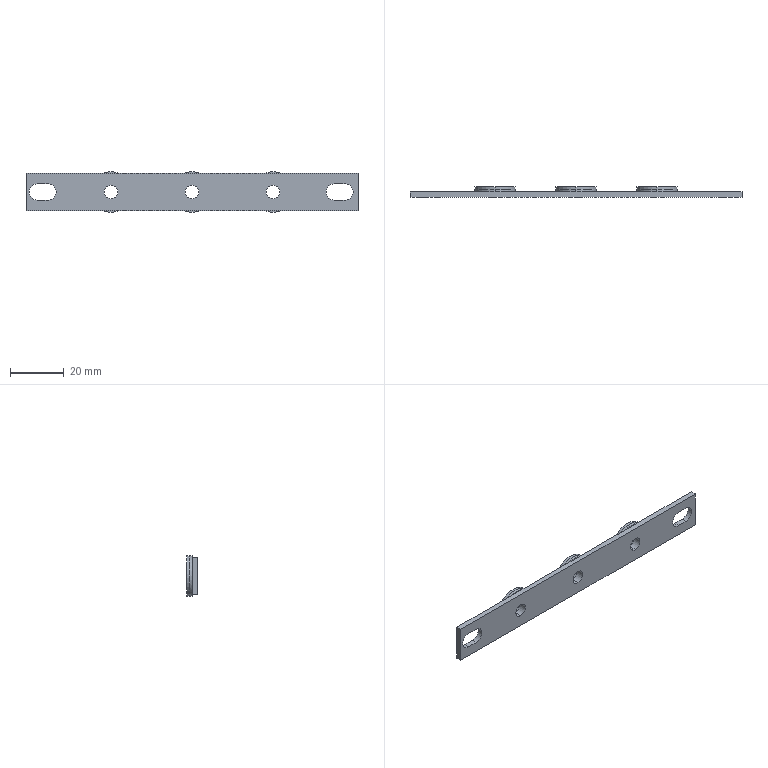Part | SolidWorks | features ICE 2, Extrusion 1 | 4 solids | 56 faces | box 123 x 4 x 15 mm | volume 4060 mm3 | cylinder 28 | plane 28 | commonest cylinder face diameters 5 x12 15 x12 6 x4